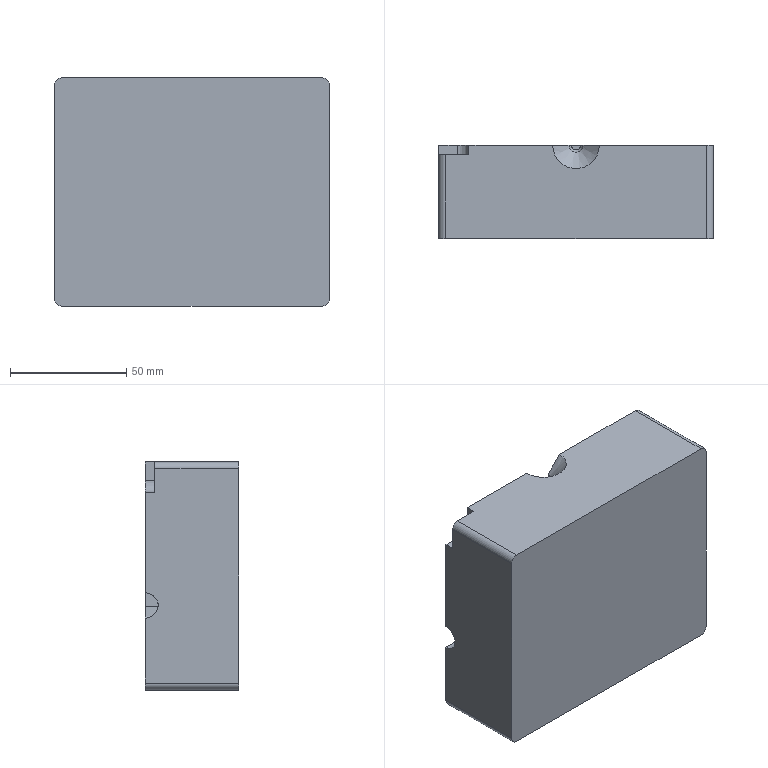NC program | NX | posted with a generic post | part box 118 x 40 x 98 mm
Lines 1 to 1487 of 39656, first 1399 of 1483 lines:
N10 G17 G21 G94 G90
(CAVITY_MILL , TOOL : D8)
N12 T00 M6
N14 G54
N16 G17 G0 G90 X63. Y44.15 S0 M3
N18 G43 Z30. H0
N20 Z-0.963
N22 G94 G1 X59. F250.
N24 X54.15
N26 Y49.
N28 X50.15
N30 Y41.
N32 G3 X51. Y40.15 R0.85
N34 G1 X59.
N36 X63.
N38 G0 Y44.15 Z-1.925
N40 G1 X59.
N42 X54.15
N44 Y49.
N46 X50.15
N48 Y41.
N50 G3 X51. Y40.15 R0.85
N52 G1 X59.
N54 X63.
N56 G0 Y44.15 Z-2.888
N58 G1 X59.
N60 X54.15
N62 Y49.
N64 X50.15
N66 Y41.
N68 G3 X51. Y40.15 R0.85
N70 G1 X59.
N72 X63.
N74 G0 Y44.15 Z-3.85
N76 G1 X59.
N78 X54.15
N80 Y49.
N82 X50.15
N84 Y41.
N86 G3 X51. Y40.15 R0.85
N88 G1 X59.
N90 X63.
N92 G0 Z30.
N94 X27.069 Y53.
N96 Z-0.963
N98 G1 Y49.
N100 Y5.639
N102 G2 X28.646 Y2.381 R4.133
N104 G1 Y-3.614
N106 X28.651 Y-3.624
N108 G2 X27.861 Y-6.049 R4.204
N110 X30.742 Y-10.011 R4.141
N112 G1 Y-17.85
N114 X31.058
N116 Y-10.
N118 G2 X33.939 Y-6.048 R4.142
N120 X33.154 Y-3.593 R4.131
N122 G1 Y2.381
N124 G2 X34.731 Y5.648 R4.173
N126 G1 Y49.
N128 Y53.
N130 G0 X27.248 Z-1.925
N132 G1 Y49.
N134 Y5.674
N136 G2 X28.872 Y2.372 R4.122
N138 G1 Y-3.614
N140 G2 X28.105 Y-6.02 R4.108
N142 X30.898 Y-8.748 R4.14
N144 X33.696 Y-6.02 R4.161
N146 X32.922 Y-3.631 R4.13
N148 G1 X32.928 Y-3.614
N150 Y2.362
N152 X32.922 Y2.376
N154 G2 X34.552 Y5.675 R4.162
N156 G1 Y48.627
N158 X34.548 Y48.99
N160 Y49.
N162 X34.549 Y53.
N164 G0 X27.557 Z-2.888
N166 G1 Y49.
N168 Y5.738
N170 G2 X29.27 Y2.372 R4.12
N172 G1 Y-3.614
N174 G2 X28.54 Y-5.964 R4.112
N176 X30.898 Y-7.482 R4.192
N178 X33.262 Y-5.964 R4.21
N180 X32.53 Y-3.614 R4.061
N182 G1 Y2.47
N184 G2 X32.736 Y3.675 R3.636
N186 X34.243 Y5.737 R4.091
N188 G1 Y48.627
N190 X34.244 Y49.
N192 X34.263 Y53.002
N194 G0 X28.029 Y53. Z-3.85
N196 G1 X28.013 Y49.
N198 X28.012 Y48.627
N200 Y5.84
N202 G2 X29.877 Y2.372 R4.129
N204 G1 Y-3.614
N206 G2 X29.204 Y-5.874 R4.028
N208 X30.9 Y-6.397 R4.605
N210 X32.594 Y-5.873 R4.686
N212 X31.923 Y-3.614 R4.073
N214 G1 Y2.372
N216 G2 X33.788 Y5.836 R4.116
N218 G1 Y49.
N220 Y53.
N222 G0 X28.649 Z-4.814
N224 G1 Y49.
N226 Y5.999
N228 G2 X30.794 Y2.372 R4.127
N230 G1 Y-3.614
N232 G2 X30.135 Y-5.85 R3.962
N234 G1 X31.665
N236 G2 X31.006 Y-3.614 R4.063
N238 G1 Y2.372
N240 G2 X33.151 Y5.997 R4.118
N242 G1 Y49.
N244 Y53.
N246 G0 X29.528 Z-5.778
N248 G1 Y49.
N250 Y6.271
N252 G2 X30.898 Y5.473 R4.416
N254 X32.272 Y6.27 R4.304
N256 G1 Y49.
N258 Y53.
N260 G0 X30.838 Z-6.742
N262 G1 X30.802 Y49.
N264 Y48.991
N266 Y6.625
N268 X30.998
N270 Y48.991
N272 Y49.
N274 X30.972 Y53.
N276 G0 Z30.
N278 X-34.726
N280 Z-0.963
N282 G1 X-34.731 Y49.
N284 Y18.094
N286 G2 X-34.817 Y17.17 R4.141
N288 G1 X-30.9 Y16.358
N290 G2 X-32.736 Y12.659 R8.141
N292 X-30.901 Y8.966 R8.142
N294 X-29.063 Y12.659 R8.158
N296 X-30.9 Y16.358 R8.143
N298 G1 X-34.817 Y17.17
N300 G2 X-38.868 Y13.869 R4.141
N302 G1 X-59.
N304 X-63.
N306 Y11.455
N308 X-59. Y11.451
N310 X-58.998
N312 X-38.907
N314 G2 X-34.731 Y7.302 R4.142
N316 G1 Y5.638
N318 G2 X-33.154 Y2.371 R4.167
N320 G1 Y-3.593
N322 G2 X-33.939 Y-6.048 R4.131
N324 X-31.058 Y-10. R4.142
N326 G1 Y-17.85
N328 X-30.742
N330 Y-10.
N332 G2 X-27.861 Y-6.049 R4.141
N334 X-28.651 Y-3.624 R4.212
N336 G1 X-28.646 Y-3.614
N338 Y2.33
N340 G2 X-27.069 Y5.627 R4.13
N342 G1 Y7.3
N344 G2 X-27.028 Y7.916 R4.615
N346 X-22.945 Y11.454 R4.158
N348 G1 X-22.932 Y11.451
N350 X-17.406
N352 G2 X-14.008 Y9.732 R4.144
N354 G1 X-10.765 Y12.074
N356 X-6.015 Y11.618
N358 X-1.702 Y11.205
N360 G2 X-1.232 Y6.796 R16.144
N362 G1 X-1.269 Y5.593
N364 G2 X0. Y5.208 R17.18
N366 X1.269 Y5.593 R17.18
N368 G1 X1.051 Y12.692
N370 G3 X-0.997 Y12.992 R1.051
N372 G2 X-1.702 Y11.205 R16.134
N374 G1 X-6.015 Y11.618
N376 G2 X-5.23 Y6.92 R12.144
N378 G1 X-5.377 Y2.148
N380 G2 X0. Y0.897 R13.18
N382 X5.377 Y2.148 R13.18
N384 G1 X5.049 Y12.815
N386 G3 X-4.797 Y14.24 R5.051
N388 G2 X-6.015 Y11.618 R12.134
N390 G1 X-10.765 Y12.074
N392 G2 X-9.228 Y7.046 R8.144
N394 G1 X-9.487 Y-1.369
N396 G2 X-9.512 Y-1.85 R10.725
N398 G1 X-5.61
N400 G2 X0. Y-3.764 R9.18
N402 X5.61 Y-1.85 R9.18
N404 G1 X9.512
N406 G2 X9.487 Y-1.369 R10.725
N408 G1 X9.047 Y12.938
N410 G3 X-8.599 Y15.485 R9.051
N412 G2 X-10.765 Y12.074 R8.134
N414 G1 X-14.008 Y9.732
N416 G2 X-13.226 Y7.172 R4.144
N418 G1 X-13.485 Y-1.246
N420 G2 X-15.508 Y-5.85 R6.725
N422 G1 X-5.61
N424 G2 X-0.525 Y-12.018 R5.18
N426 G1 X-3.027 Y-24.888
N428 X-1.75
N430 G2 X0. Y-25.269 R4.155
N432 X1.751 Y-24.888 R4.178
N434 G1 X3.027
N436 X0.525 Y-12.018
N438 G2 X5.61 Y-5.85 R5.18
N440 G1 X15.508
N442 G2 X13.485 Y-1.246 R6.725
N444 G1 X13.045 Y13.061
N446 G3 X-12.401 Y16.727 R13.051
N448 G2 X-16.352 Y13.869 R4.134
N450 G1 X-22.932
N452 G2 X-27.069 Y18.094 R4.143
N454 G1 Y49.
N456 Y53.
N458 G0 X-34.542 Z-1.925
N460 G1 X-34.552 Y49.
N462 Y18.094
N464 X-34.551 Y17.754
N466 G2 X-34.728 Y16.533 R4.134
N468 G1 X-30.899 Y15.375
N470 G2 X-32.325 Y12.659 R8.134
N472 X-30.9 Y9.946 R8.135
N474 X-29.475 Y12.662 R8.133
N476 X-29.772 Y13.057 R8.36
N478 X-30.899 Y15.375 R8.194
N480 G1 X-34.728 Y16.533
N482 G2 X-38.673 Y13.595 R4.134
N484 G1 X-59.
N486 X-63.
N488 Y11.727
N490 X-59. Y11.725
N492 X-58.993
N494 X-38.687
N496 G2 X-34.552 Y7.589 R4.135
N498 G1 Y5.664
N500 G2 X-32.928 Y2.371 R4.126
N502 G1 Y-3.614
N504 X-32.922 Y-3.631
N506 G2 X-33.695 Y-6.019 R4.131
N508 X-30.902 Y-8.75 R4.141
N510 X-28.105 Y-6.02 R4.157
N512 X-28.872 Y-3.614 R4.111
N514 G1 Y2.362
N516 G2 X-27.248 Y5.663 R4.117
N518 G1 Y7.592
N520 G2 X-23.116 Y11.725 R4.133
N522 G1 X-17.391
N524 G2 X-13.906 Y9.869 R4.147
N526 G1 X-10.572 Y12.08
N528 X-5.919 Y11.653
N530 X-1.641 Y11.26
N532 G2 X-1.224 Y7.055 R16.147
N534 G1 X-1.269 Y5.597
N536 G2 X0.004 Y5.213 R17.18
N538 X1.269 Y5.595 R17.187
N540 G1 X1.051 Y12.692
N542 G3 X-1.002 Y12.976 R1.051
N544 G2 X-1.641 Y11.26 R16.147
N546 G1 X-5.919 Y11.653
N548 G2 X-5.222 Y7.182 R12.147
N550 G1 X-5.377 Y2.148
N552 G2 X0.004 Y0.903 R13.18
N554 X5.377 Y2.148 R13.187
N556 G1 X5.049 Y12.815
N558 G3 X-4.822 Y14.162 R5.051
N560 G2 X-5.919 Y11.653 R12.147
N562 G1 X-10.572 Y12.08
N564 G2 X-9.22 Y7.309 R8.147
N566 G1 X-9.487 Y-1.369
N568 G2 X-9.512 Y-1.85 R10.725
N570 G1 X-5.593
N572 G2 X0.003 Y-3.753 R9.18
N574 X5.59 Y-1.85 R9.187
N576 G1 X9.512
N578 G2 X9.487 Y-1.369 R10.725
N580 G1 X9.047 Y12.938
N582 G3 X-8.644 Y15.345 R9.051
N584 G2 X-10.572 Y12.08 R8.147
N586 G1 X-13.906 Y9.869
N588 G2 X-13.218 Y7.437 R4.147
N590 G1 X-13.485 Y-1.246
N592 G2 X-15.508 Y-5.85 R6.725
N594 G1 X-5.593
N596 G2 X-0.508 Y-12.018 R5.18
N598 G1 X-3.006 Y-24.871
N600 X-0.532
N602 X-0.174 Y-24.879
N604 X0. Y-24.89
N606 G2 X0.529 Y-24.871 R5.99
N608 G1 X3.006
N610 X0.511 Y-12.036
N612 G2 X5.593 Y-5.85 R5.187
N614 G1 X15.508
N616 G2 X13.485 Y-1.246 R6.725
N618 G1 X13.045 Y13.061
N620 G3 X-12.465 Y16.526 R13.051
N622 G2 X-16.436 Y13.595 R4.147
N624 G1 X-23.119
N626 G2 X-25.166 Y14.136 R4.14
N628 X-26.502 Y15.36 R4.36
N630 X-27.246 Y17.528 R4.194
N632 G1 X-27.248 Y18.094
N634 Y49.
N636 Y53.
N638 G0 X-34.243 Z-2.888
N640 G1 Y49.
N642 Y17.237
N644 G2 X-34.485 Y15.832 R4.195
N646 X-34.576 Y15.599 R4.12
N648 G1 X-30.899 Y14.025
N650 G2 X-31.647 Y12.659 R8.12
N652 X-30.901 Y11.295 R8.131
N654 X-30.153 Y12.661 R8.123
N656 X-30.899 Y14.025 R8.133
N658 G1 X-34.576 Y15.599
N660 G2 X-38.401 Y13.101 R4.12
N662 G1 X-59.
N664 X-63.
N666 Y12.219
N668 X-59.
N670 X-38.907
N672 X-38.343 Y12.222
N674 G2 X-34.243 Y8.076 R4.131
N676 G1 Y5.728
N678 G2 X-32.838 Y3.958 R4.254
N680 G1 X-32.698 Y3.537
N682 G2 X-32.53 Y2.499 R3.292
N684 G1 Y-3.614
N686 G2 X-33.261 Y-5.964 R4.061
N688 X-30.902 Y-7.482 R4.17
N690 X-28.544 Y-5.965 R4.243
N692 X-29.27 Y-3.614 R4.166
N694 G1 Y2.362
N696 G2 X-27.557 Y5.727 R4.119
N698 G1 Y8.077
N700 G2 X-23.395 Y12.219 R4.123
N702 G1 X-17.313
N704 G2 X-13.815 Y10.235 R4.119
N706 G1 X-13.783 Y10.178
N708 X-13.75 Y10.12
N710 X-10.272 Y12.097
N712 X-5.766 Y11.715
N714 X-1.543 Y11.358
N716 G2 X-1.209 Y7.542 R16.2
N718 G1 X-1.269 Y5.601
N720 G2 X0.004 Y5.219 R17.18
N722 X1.269 Y5.599 R17.187
N724 G1 X1.051 Y12.692
N726 G3 X-1.012 Y12.943 R1.051
N728 G2 X-1.543 Y11.358 R16.201
N730 G1 X-5.766 Y11.715
N732 G2 X-5.207 Y7.666 R12.2
N734 G1 X-5.377 Y2.148
N736 G2 X0.004 Y0.911 R13.18
N738 X5.377 Y2.148 R13.187
N740 G1 X5.049 Y12.815
N742 G3 X-4.865 Y14.018 R5.051
N744 G2 X-5.766 Y11.715 R12.201
N746 G1 X-10.272 Y12.097
N748 G2 X-9.205 Y7.79 R8.2
N750 G1 X-9.487 Y-1.369
N752 G2 X-9.512 Y-1.85 R10.725
N754 G1 X-5.576
N756 G2 X0.003 Y-3.74 R9.18
N758 X5.572 Y-1.85 R9.187
N760 G1 X9.512
N762 G2 X9.487 Y-1.369 R10.725
N764 G1 X9.047 Y12.938
N766 G3 X-8.718 Y15.091 R9.051
N768 G2 X-10.272 Y12.097 R8.201
N770 G1 X-13.75 Y10.12
N772 G2 X-13.203 Y7.914 R4.2
N774 G1 X-13.485 Y-1.246
N776 G2 X-15.508 Y-5.85 R6.725
N778 G1 X-5.576
N780 G2 X-0.491 Y-12.018 R5.18
N782 G1 X-2.986 Y-24.855
N784 X2.986
N786 X0.494 Y-12.036
N788 G2 X5.576 Y-5.85 R5.187
N790 G1 X15.508
N792 G2 X13.485 Y-1.246 R6.725
N794 G1 X13.045 Y13.061
N796 G3 X-12.572 Y16.164 R13.051
N798 G2 X-16.07 Y13.125 R4.201
N800 G1 X-16.596 Y13.094
N802 X-16.614 Y13.101
N804 X-23.44
N806 G2 X-25.703 Y13.781 R4.105
N808 X-27.557 Y17.229 R4.133
N810 G1 Y49.
N812 Y53.
N814 G0 Z30.
N816 X-2.563 Y12.197
N818 Z-2.388
N820 G3 X-2.563 Y12.197 Z-2.607 I1.979 J-0.286
N822 X-2.563 Y12.197 Z-2.826 I1.979 J-0.286
N824 X-2.563 Y12.197 Z-3.046 I1.979 J-0.286
N826 X-2.563 Y12.197 Z-3.265 I1.979 J-0.286
N828 X-2.563 Y12.197 Z-3.484 I1.979 J-0.286
N830 X-2.563 Y12.197 Z-3.704 I1.979 J-0.286
N832 X0.646 Y13.489 Z-3.85 R-2.
N834 X-0.473 Y13.598 R1.051
N836 X-1.027 Y12.883 R1.051
N838 G2 X-1.407 Y11.517 R16.402
N840 X-1.184 Y8.341 R16.452
N842 G1 X-1.269 Y5.606
N844 G2 X0.004 Y5.225 R17.18
N846 X1.269 Y5.604 R17.187
N848 G1 X1.051 Y12.692
N850 G3 X0.646 Y13.489 R1.051
N852 G1 X3.104 Y16.645
N854 G3 X-2.274 Y17.17 R5.051
N856 X-4.925 Y13.779 R5.051
N858 G2 X-5.555 Y11.824 R12.402
N860 X-5.183 Y8.456 R12.452
N862 G1 X-5.377 Y2.149
N864 G2 X0.004 Y0.919 R13.18
N866 X5.377 Y2.149 R13.187
N868 G1 X5.049 Y12.815
N870 G3 X3.104 Y16.645 R5.051
N872 G1 X5.562 Y19.801
N874 G3 X-8.823 Y14.68 R9.051
N876 G2 X-9.876 Y12.144 R8.402
N878 X-9.603 Y11.429 R8.123
N880 X-9.181 Y8.568 R8.452
N882 G1 X-9.487 Y-1.369
N884 G2 X-9.512 Y-1.85 R10.725
N886 G1 X-5.559
N888 G2 X0.003 Y-3.727 R9.18
N890 X5.555 Y-1.85 R9.187
N892 G1 X9.512
N894 G2 X9.487 Y-1.369 R10.725
N896 G1 X9.047 Y12.938
N898 G3 X5.562 Y19.801 R9.051
N900 G1 X8.02 Y22.956
N902 G3 X-12.719 Y15.585 R13.051
N904 G2 X-13.533 Y13.884 R4.402
N906 X-15.407 Y12.542 R4.123
N908 X-13.402 Y10.178 R4.123
N910 X-13.18 Y8.678 R4.452
N912 G1 X-13.485 Y-1.246
N914 G2 X-15.508 Y-5.85 R6.725
N916 G1 X-5.559
N918 G2 X-0.474 Y-12.018 R5.18
N920 G1 X-2.966 Y-24.838
N922 X2.966
N924 X0.477 Y-12.036
N926 G2 X5.559 Y-5.85 R5.187
N928 G1 X15.508
N930 G2 X13.485 Y-1.246 R6.725
N932 G1 X13.045 Y13.061
N934 G3 X8.02 Y22.956 R13.051
N936 G1 X7.036 Y21.694
N938 G0 X-2.547 Y12.291 Z-3.35
N940 G3 X-2.547 Y12.291 Z-3.569 I1.964 J-0.38
N942 X-2.547 Y12.291 Z-3.789 I1.964 J-0.38
N944 X-2.547 Y12.291 Z-4.008 I1.964 J-0.38
N946 X-2.547 Y12.291 Z-4.227 I1.964 J-0.38
N948 X-2.547 Y12.291 Z-4.447 I1.964 J-0.38
N950 X-2.547 Y12.291 Z-4.666 I1.964 J-0.38
N952 X0.646 Y13.489 Z-4.814 R-2.
N954 X-1.039 Y12.818 R1.051
N956 G2 X-1.221 Y11.81 R16.601
N958 X-1.146 Y9.601 R16.541
N960 G1 X-1.268 Y5.61
N962 G2 X0.004 Y5.23 R17.18
N964 X1.268 Y5.608 R17.187
N966 G1 X1.051 Y12.692
N968 G3 X0.646 Y13.489 R1.051
N970 G1 X3.104 Y16.645
N972 G3 X-4.995 Y13.411 R5.051
N974 G2 X-5.28 Y12.03 R12.601
N976 X-5.144 Y9.728 R12.541
N978 G1 X-5.377 Y2.149
N980 G2 X0.004 Y0.927 R13.18
N982 X5.377 Y2.149 R13.187
N984 G1 X5.049 Y12.815
N986 G3 X3.104 Y16.645 R5.051
N988 G1 X5.562 Y19.801
N990 G3 X-8.951 Y14.002 R9.051
N992 G2 X-9.403 Y12.253 R8.601
N994 X-9.142 Y9.855 R8.541
N996 G1 X-9.487 Y-1.369
N998 G2 X-9.512 Y-1.85 R10.725
N1000 G1 X-5.542
N1002 G2 X0.003 Y-3.714 R9.18
N1004 X5.538 Y-1.85 R9.187
N1006 G1 X9.512
N1008 G2 X9.487 Y-1.369 R10.725
N1010 G1 X9.047 Y12.938
N1012 G3 X5.562 Y19.801 R9.051
N1014 G1 X8.02 Y22.956
N1016 G3 X-12.907 Y14.592 R13.051
N1018 G2 X-13.791 Y12.488 R4.601
N1020 X-13.139 Y9.984 R4.541
N1022 G1 X-13.485 Y-1.246
N1024 G2 X-15.508 Y-5.85 R6.725
N1026 G1 X-5.542
N1028 G2 X-0.457 Y-12.018 R5.18
N1030 G1 X-2.945 Y-24.821
N1032 X2.945
N1034 X0.46 Y-12.036
N1036 G2 X5.542 Y-5.85 R5.187
N1038 G1 X15.508
N1040 G2 X13.485 Y-1.246 R6.725
N1042 G1 X13.045 Y13.061
N1044 G3 X8.02 Y22.956 R13.051
N1046 G1 X7.036 Y21.694
N1048 G0 X-2.547 Y12.291 Z-4.314
N1050 G3 X-2.547 Y12.291 Z-4.534 I1.964 J-0.38
N1052 X-2.547 Y12.291 Z-4.753 I1.964 J-0.38
N1054 X-2.547 Y12.291 Z-4.972 I1.964 J-0.38
N1056 X-2.547 Y12.291 Z-5.192 I1.964 J-0.38
N1058 X-2.547 Y12.291 Z-5.411 I1.964 J-0.38
N1060 X-2.547 Y12.291 Z-5.63 I1.964 J-0.38
N1062 X0.646 Y13.489 Z-5.778 R-2.
N1064 X-1.051 Y12.692 R1.051
N1066 G1 X-1.268 Y5.614
N1068 G2 X0.004 Y5.236 R17.18
N1070 X1.268 Y5.612 R17.187
N1072 G1 X1.051 Y12.692
N1074 G3 X0.646 Y13.489 R1.051
N1076 G1 X3.104 Y16.645
N1078 G3 X-5.049 Y12.815 R5.051
N1080 G1 X-5.377 Y2.149
N1082 G2 X0.004 Y0.935 R13.18
N1084 X5.377 Y2.149 R13.187
N1086 G1 X5.049 Y12.815
N1088 G3 X3.104 Y16.645 R5.051
N1090 G1 X5.562 Y19.801
N1092 G3 X-9.047 Y12.938 R9.051
N1094 G1 X-9.487 Y-1.369
N1096 G2 X-9.512 Y-1.85 R10.725
N1098 G1 X-5.524
N1100 G2 X0.003 Y-3.701 R9.18
N1102 X5.521 Y-1.85 R9.187
N1104 G1 X9.512
N1106 G2 X9.487 Y-1.369 R10.725
N1108 G1 X9.047 Y12.938
N1110 G3 X5.562 Y19.801 R9.051
N1112 G1 X8.02 Y22.956
N1114 G3 X-13.045 Y13.061 R13.051
N1116 G1 X-13.485 Y-1.246
N1118 G2 X-15.508 Y-5.85 R6.725
N1120 G1 X-5.524
N1122 G2 X-0.439 Y-12.018 R5.18
N1124 G1 X-2.925 Y-24.804
N1126 X2.925
N1128 X0.443 Y-12.036
N1130 G2 X5.524 Y-5.85 R5.187
N1132 G1 X15.508
N1134 G2 X13.485 Y-1.246 R6.725
N1136 G1 X13.045 Y13.061
N1138 G3 X8.02 Y22.956 R13.051
N1140 G1 X7.036 Y21.694
N1142 G0 X-2.547 Y12.291 Z-5.278
N1144 G3 X-2.547 Y12.291 Z-5.498 I1.964 J-0.38
N1146 X-2.547 Y12.291 Z-5.717 I1.964 J-0.38
N1148 X-2.547 Y12.291 Z-5.936 I1.964 J-0.38
N1150 X-2.547 Y12.291 Z-6.156 I1.964 J-0.38
N1152 X-2.547 Y12.291 Z-6.375 I1.964 J-0.38
N1154 X-2.547 Y12.291 Z-6.594 I1.964 J-0.38
N1156 X0.646 Y13.489 Z-6.742 R-2.
N1158 X-1.051 Y12.692 R1.051
N1160 G1 X-1.268 Y5.619
N1162 G2 X0.004 Y5.242 R17.18
N1164 X1.268 Y5.617 R17.187
N1166 G1 X1.051 Y12.692
N1168 G3 X0.646 Y13.489 R1.051
N1170 G1 X3.104 Y16.645
N1172 G3 X-5.049 Y12.815 R5.051
N1174 G1 X-5.377 Y2.149
N1176 G2 X0.004 Y0.943 R13.18
N1178 X5.377 Y2.149 R13.187
N1180 G1 X5.049 Y12.815
N1182 G3 X3.104 Y16.645 R5.051
N1184 G1 X5.562 Y19.801
N1186 G3 X-9.047 Y12.938 R9.051
N1188 G1 X-9.487 Y-1.369
N1190 G2 X-9.512 Y-1.85 R10.725
N1192 G1 X-5.507
N1194 G2 X0.003 Y-3.688 R9.18
N1196 X5.504 Y-1.85 R9.187
N1198 G1 X9.512
N1200 G2 X9.487 Y-1.369 R10.725
N1202 G1 X9.047 Y12.938
N1204 G3 X5.562 Y19.801 R9.051
N1206 G1 X8.02 Y22.956
N1208 G3 X-13.045 Y13.061 R13.051
N1210 G1 X-13.485 Y-1.246
N1212 G2 X-15.508 Y-5.85 R6.725
N1214 G1 X-5.507
N1216 G2 X-0.422 Y-12.018 R5.18
N1218 G1 X-2.904 Y-24.787
N1220 X2.904
N1222 X0.426 Y-12.036
N1224 G2 X5.507 Y-5.85 R5.187
N1226 G1 X15.508
N1228 G2 X13.485 Y-1.246 R6.725
N1230 G1 X13.045 Y13.061
N1232 G3 X8.02 Y22.956 R13.051
N1234 G1 X7.036 Y21.694
N1236 G0 X-2.547 Y12.291 Z-6.242
N1238 G3 X-2.547 Y12.291 Z-6.462 I1.964 J-0.38
N1240 X-2.547 Y12.291 Z-6.681 I1.964 J-0.38
N1242 X-2.547 Y12.291 Z-6.901 I1.964 J-0.38
N1244 X-2.547 Y12.291 Z-7.12 I1.964 J-0.38
N1246 X-2.547 Y12.291 Z-7.339 I1.964 J-0.38
N1248 X-2.547 Y12.291 Z-7.559 I1.964 J-0.38
N1250 X0.646 Y13.489 Z-7.707 R-2.
N1252 X-1.051 Y12.692 R1.051
N1254 G1 X-1.268 Y5.625
N1256 G2 X0.002 Y5.25 R17.184
N1258 X1.268 Y5.623 R17.18
N1260 G1 X1.051 Y12.692
N1262 G3 X0.646 Y13.489 R1.051
N1264 G1 X3.104 Y16.645
N1266 G3 X-5.049 Y12.815 R5.051
N1268 G1 X-5.377 Y2.15
N1270 X-5.234
N1272 G2 X0.001 Y0.953 R13.184
N1274 X5.377 Y2.15 R13.18
N1276 G1 X5.049 Y12.815
N1278 G3 X3.104 Y16.645 R5.051
N1280 G1 X5.562 Y19.801
N1282 G3 X-9.047 Y12.938 R9.051
N1284 G1 X-9.487 Y-1.369
N1286 G2 X-9.512 Y-1.85 R10.725
N1288 G1 X-5.28
N1290 G2 X0. Y-3.673 R9.184
N1292 X5.49 Y-1.85 R9.18
N1294 G1 X9.512
N1296 G2 X9.487 Y-1.369 R10.725
N1298 G1 X9.047 Y12.938
N1300 G3 X5.562 Y19.801 R9.051
N1302 G1 X8.02 Y22.956
N1304 G3 X-13.045 Y13.061 R13.051
N1306 G1 X-13.485 Y-1.246
N1308 G2 X-15.508 Y-5.85 R6.725
N1310 G1 X-5.34
N1312 G2 X-0.405 Y-12.018 R5.184
N1314 G1 X-2.884 Y-24.77
N1316 X2.884
N1318 X0.405 Y-12.018
N1320 G2 X5.49 Y-5.85 R5.18
N1322 G1 X15.508
N1324 G2 X13.485 Y-1.246 R6.725
N1326 G1 X13.045 Y13.061
N1328 G3 X8.02 Y22.956 R13.051
N1330 G1 X7.036 Y21.694
N1332 G0 X-2.555 Y12.281 Z-7.207
N1334 G3 X-2.555 Y12.281 Z-7.426 I1.964 J-0.38
N1336 X-2.555 Y12.281 Z-7.645 I1.964 J-0.38
N1338 X-2.555 Y12.281 Z-7.865 I1.964 J-0.38
N1340 X-2.555 Y12.281 Z-8.084 I1.964 J-0.38
N1342 X-2.555 Y12.281 Z-8.303 I1.964 J-0.38
N1344 X-2.555 Y12.281 Z-8.523 I1.964 J-0.38
N1346 X0.638 Y13.479 Z-8.671 R-2.
N1348 X-1.037 Y12.692 R1.038
N1350 G1 X-1.255 Y5.627
N1352 G2 X0.001 Y5.257 R17.193
N1354 X1.255 Y5.626 R17.18
N1356 G1 X1.037 Y12.692
N1358 G3 X0.638 Y13.479 R1.038
N1360 G1 X3.096 Y16.634
N1362 G3 X-5.035 Y12.815 R5.038
N1364 G1 X-5.363 Y2.15
N1366 X-5.193
N1368 G2 X0. Y0.963 R13.193
N1370 X5.363 Y2.15 R13.18
N1372 G1 X5.035 Y12.815
N1374 G3 X3.096 Y16.634 R5.038
N1376 G1 X5.553 Y19.79
N1378 G3 X-9.033 Y12.938 R9.038
N1380 G1 X-9.473 Y-1.345
N1382 G2 X-9.496 Y-1.85 R10.004
N1384 G1 X-5.243
N1386 G2 X-0.001 Y-3.655 R9.193
N1388 X5.472 Y-1.85 R9.18
N1390 G1 X9.496
N1392 G2 X9.471 Y-1.367 R10.699
N1394 G1 X9.469 Y-1.217
N1396 X9.033 Y12.938
N1398 G3 X5.553 Y19.79 R9.038
N1400 G1 X8.011 Y22.946
N1402 G3 X-13.032 Y13.061 R13.038
N1404 G1 X-13.472 Y-1.245
N1406 G2 X-13.561 Y-2.175 R6.004
N1408 X-15.493 Y-5.85 R6.758
N1410 G1 X-5.308
N1412 G2 X-0.366 Y-11.968 R5.193
N1414 G1 X-0.383 Y-12.017
N1416 X-2.857 Y-24.749
N1418 X2.857
N1420 X0.402 Y-12.116
N1422 G2 X5.471 Y-5.85 R5.18
N1424 G1 X15.497
N1426 G2 X13.469 Y-1.247 R6.699
N1428 G1 X13.472 Y-1.245
N1430 X13.032 Y13.061
N1432 G3 X8.011 Y22.946 R13.038
N1434 G1 X7.028 Y21.684
N1436 G0 Z30.
N1438 X-0.383 Y-23.247
N1440 Z-8.171
N1442 G3 X-0.383 Y-23.247 Z-8.311 I0.383 J1.221
N1444 X-0.383 Y-23.247 Z-8.452 I0.383 J1.221
N1446 X-0.383 Y-23.247 Z-8.592 I0.383 J1.221
N1448 X-0.383 Y-23.247 Z-8.732 I0.383 J1.221
N1450 X-0.383 Y-23.247 Z-8.873 I0.383 J1.221
N1452 X-0.383 Y-23.247 Z-9.013 I0.383 J1.221
N1454 X-0.383 Y-23.247 Z-9.154 I0.383 J1.221
N1456 X-0.383 Y-23.247 Z-9.294 I0.383 J1.221
N1458 X-0.383 Y-23.247 Z-9.434 I0.383 J1.221
N1460 X-0.383 Y-23.247 Z-9.575 I0.383 J1.221
N1462 X0.868 Y-21.085 Z-9.635 R1.28
N1464 G1 X-0.819 Y-19.531
N1466 X-1.638 Y-23.743
N1468 X1.638
N1470 X0. Y-15.318
N1472 X-0.819 Y-19.531
N1474 X0.752 Y-19.836
N1476 G0 Z30.
N1478 X-2.801 Y11.965
N1480 Z-8.171
N1482 G3 X-2.801 Y11.965 Z-8.39 I1.964 J-0.38
N1484 X-2.801 Y11.965 Z-8.61 I1.964 J-0.38
N1486 X-2.801 Y11.965 Z-8.829 I1.964 J-0.38
N1488 X-2.801 Y11.965 Z-9.048 I1.964 J-0.38
N1490 X-2.801 Y11.965 Z-9.268 I1.964 J-0.38
N1492 X-2.801 Y11.965 Z-9.487 I1.964 J-0.38
N1494 X0.392 Y13.163 Z-9.635 R-2.
N1496 X-0.637 Y12.68 R0.638
N1498 G1 X-0.855 Y5.609
N1500 G2 X0. Y5.37 R17.834
N1502 X0.855 Y5.609 R17.828
N1504 G1 X0.637 Y12.68
N1506 G3 X0.392 Y13.163 R0.638
N1508 G1 X2.85 Y16.319
N1510 G3 X-4.636 Y12.803 R4.638
N1512 G1 X-4.963 Y2.148
N1514 G2 X0. Y1.129 R13.834
N1516 X4.963 Y2.148 R13.828
N1518 G1 X4.636 Y12.803
N1520 G3 X2.85 Y16.319 R4.638
N1522 G1 X5.308 Y19.475
N1524 G3 X-8.634 Y12.926 R8.638
N1526 G1 X-9.086 Y-1.78
N1528 X-9.088 Y-1.85
N1530 X-5.186
N1532 G2 X-0.688 Y-2.954 R9.834
N1534 X0.001 Y-3.344 R11.752
N1536 X0.684 Y-2.956 R11.722
N1538 X5.185 Y-1.85 R9.828
N1540 G1 X9.088
N1542 X9.086 Y-1.778
N1544 X8.634 Y12.926
N1546 G3 X5.308 Y19.475 R8.638
N1548 G1 X7.766 Y22.63
N1550 G3 X-12.632 Y13.049 R12.638
N1552 G1 X-13.085 Y-1.68
N1554 G2 X-14.862 Y-5.85 R6.027
N1556 G1 X-5.193
N1558 G2 X-2.534 Y-6.502 R5.834
N1560 X0.007 Y-8.632 R7.752
N1562 X2.535 Y-6.502 R7.722
N1564 X5.192 Y-5.85 R5.828
N1566 G1 X14.864
N1568 G2 X13.085 Y-1.68 R6.012
N1570 G1 X12.632 Y13.049
N1572 G3 X7.766 Y22.63 R12.638
N1574 G1 X6.782 Y21.368
N1576 G0 X0.4 Y6.509 Z-9.135
N1578 G3 X0.4 Y6.509 Z-9.354 I-1.802 J0.868
N1580 X0.4 Y6.509 Z-9.574 I-1.802 J0.868
N1582 X0.4 Y6.509 Z-9.793 I-1.802 J0.868
N1584 X0.4 Y6.509 Z-10.012 I-1.802 J0.868
N1586 X0.4 Y6.509 Z-10.232 I-1.802 J0.868
N1588 X-3.401 Y7.438 Z-10.356 R-2.
N1590 G1 X-3.565 Y2.117
N1592 G2 X-2.825 Y2.058 R19.124
N1594 G1 X-0.002 Y2.057
N1596 X2.838 Y2.059
N1598 G2 X3.565 Y2.117 R19.215
N1600 G1 X3.237 Y12.76
N1602 G3 X-3.237 Y12.76 R3.239
N1604 G1 X-3.401 Y7.438
N1606 X-7.399 Y7.561
N1608 X-7.688 Y-1.85
N1610 X-4.535
N1612 G2 X-3.059 Y-1.939 R15.124
N1614 G1 X-3.004 Y-1.942
N1616 X-0.001 Y-1.943
N1618 X3.012 Y-1.941
N1620 X3.069 Y-1.938
N1622 G2 X4.534 Y-1.85 R15.215
N1624 G1 X7.688
N1626 X7.235 Y12.883
N1628 G3 X-7.235 Y12.883 R7.239
N1630 G1 X-7.399 Y7.561
N1632 X-11.397 Y7.684
N1634 X-11.728 Y-3.069
N1636 G2 X-12.88 Y-5.85 R4.292
N1638 G1 X-4.561
N1640 G2 X-3.383 Y-5.928 R11.124
N1642 G1 X-3.102 Y-5.942
N1644 X0. Y-5.943
N1646 X3.102 Y-5.941
N1648 X3.383 Y-5.928
N1650 G2 X4.561 Y-5.85 R11.215
N1652 G1 X12.873
N1654 G2 X11.728 Y-3.069 R4.164
N1656 G1 X11.233 Y13.006
N1658 G3 X-11.233 Y13.006 R11.239
N1660 G1 X-11.397 Y7.684
N1662 X-9.798 Y7.635
N1664 G0 Z30.
N1666 X-33.788 Y53.
N1668 Z-3.85
N1670 G1 Y49.
N1672 Y16.441
N1674 G2 X-36.224 Y12.661 R4.113
N1676 X-33.836 Y9.506 R4.097
N1678 X-33.788 Y8.839 R4.657
N1680 G1 Y5.829
N1682 G2 X-31.923 Y2.362 R4.126
N1684 G1 Y-3.614
N1686 G2 X-32.594 Y-5.874 R4.077
N1688 X-30.9 Y-6.397 R4.674
N1690 X-29.207 Y-5.875 R4.643
N1692 X-29.877 Y-3.614 R4.069
N1694 G1 Y2.362
N1696 G2 X-28.012 Y5.826 R4.112
N1698 G1 Y8.806
N1700 G2 X-27.918 Y9.748 R4.772
N1702 X-25.576 Y12.658 R4.052
N1704 X-27.989 Y16.049 R4.094
N1706 X-28.012 Y16.58 R6.243
N1708 G1 Y49.
N1710 Y53.
N1712 G0 X-33.151 Z-4.814
N1714 G1 Y49.
N1716 Y15.027
N1718 G2 X-33.866 Y12.66 R4.229
N1720 X-33.151 Y10.292 R4.218
N1722 G1 Y5.991
N1724 G2 X-31.006 Y2.362 R4.139
N1726 G1 Y-3.614
N1728 G2 X-31.665 Y-5.85 R4.063
N1730 G1 X-30.135
N1732 G2 X-30.794 Y-3.614 R3.964
N1734 G1 Y2.362
N1736 G2 X-28.649 Y5.99 R4.13
N1738 G1 Y10.293
N1740 G2 X-27.933 Y12.66 R4.252
N1742 X-28.649 Y15.028 R4.254
N1744 G1 Y49.
N1746 Y53.
N1748 G0 X-32.272 Z-5.778
N1750 G1 Y49.
N1752 Y6.259
N1754 G2 X-30.9 Y5.462 R4.151
N1756 X-29.528 Y6.259 R4.357
N1758 G1 Y49.
N1760 Y53.
N1762 G0 X-30.998 Z-6.742
N1764 G1 Y49.
N1766 Y6.615
N1768 X-30.802
N1770 Y49.
N1772 Y53.
N1774 G0 Z30.
N1776 X-50.75 Y38.985
N1778 Z0.5
N1780 G3 X-50.75 Y38.985 Z0.308 I1.75 J0.015
N1782 X-50.75 Y38.985 Z0.116 I1.75 J0.015
N1784 X-50.75 Y38.985 Z-0.076 I1.75 J0.015
N1786 X-50.75 Y38.985 Z-0.268 I1.75 J0.015
N1788 X-50.75 Y38.985 Z-0.46 I1.75 J0.015
N1790 X-50.75 Y38.985 Z-0.652 I1.75 J0.015
N1792 X-50.75 Y38.985 Z-0.844 I1.75 J0.015
N1794 X-47.735 Y40.209 Z-0.963 R-1.75
N1796 X-50.209 Y40.265 R1.75
N1798 X-47.735 Y40.209 R-1.75
N1800 G1 X-48.892 Y39.104
N1802 G0 X-50.75 Y38.985 Z-0.463
N1804 G3 X-50.75 Y38.985 Z-0.654 I1.75 J0.015
N1806 X-50.75 Y38.985 Z-0.846 I1.75 J0.015
N1808 X-50.75 Y38.985 Z-1.038 I1.75 J0.015
N1810 X-50.75 Y38.985 Z-1.23 I1.75 J0.015
N1812 X-50.75 Y38.985 Z-1.422 I1.75 J0.015
N1814 X-50.75 Y38.985 Z-1.614 I1.75 J0.015
N1816 X-50.75 Y38.985 Z-1.806 I1.75 J0.015
N1818 X-47.735 Y40.209 Z-1.925 R-1.75
N1820 X-50.209 Y40.265 R1.75
N1822 X-47.735 Y40.209 R-1.75
N1824 G1 X-48.892 Y39.104
N1826 G0 X-50.75 Y38.985 Z-1.425
N1828 G3 X-50.75 Y38.985 Z-1.617 I1.75 J0.015
N1830 X-50.75 Y38.985 Z-1.809 I1.75 J0.015
N1832 X-50.75 Y38.985 Z-2.001 I1.75 J0.015
N1834 X-50.75 Y38.985 Z-2.193 I1.75 J0.015
N1836 X-50.75 Y38.985 Z-2.385 I1.75 J0.015
N1838 X-50.75 Y38.985 Z-2.577 I1.75 J0.015
N1840 X-50.75 Y38.985 Z-2.769 I1.75 J0.015
N1842 X-47.735 Y40.209 Z-2.888 R-1.75
N1844 X-50.209 Y40.265 R1.75
N1846 X-47.735 Y40.209 R-1.75
N1848 G1 X-48.892 Y39.104
N1850 G0 X-50.75 Y38.985 Z-2.388
N1852 G3 X-50.75 Y38.985 Z-2.579 I1.75 J0.015
N1854 X-50.75 Y38.985 Z-2.771 I1.75 J0.015
N1856 X-50.75 Y38.985 Z-2.963 I1.75 J0.015
N1858 X-50.75 Y38.985 Z-3.155 I1.75 J0.015
N1860 X-50.75 Y38.985 Z-3.347 I1.75 J0.015
N1862 X-50.75 Y38.985 Z-3.539 I1.75 J0.015
N1864 X-50.75 Y38.985 Z-3.731 I1.75 J0.015
N1866 X-47.735 Y40.209 Z-3.85 R-1.75
N1868 X-50.209 Y40.265 R1.75
N1870 X-47.735 Y40.209 R-1.75
N1872 G1 X-48.892 Y39.104
N1874 G0 X-50.748 Y39.08 Z-3.35
N1876 G3 X-50.748 Y39.08 Z-3.542 I1.748 J-0.08
N1878 X-50.748 Y39.08 Z-3.734 I1.748 J-0.08
N1880 X-50.748 Y39.08 Z-3.926 I1.748 J-0.08
N1882 X-50.748 Y39.08 Z-4.118 I1.748 J-0.08
N1884 X-50.748 Y39.08 Z-4.31 I1.748 J-0.08
N1886 X-50.748 Y39.08 Z-4.502 I1.748 J-0.08
N1888 X-50.748 Y39.08 Z-4.694 I1.748 J-0.08
N1890 X-47.735 Y40.209 Z-4.814 R-1.75
N1892 X-50.209 Y40.265 R1.75
N1894 X-47.735 Y40.209 R-1.75
N1896 G1 X-48.892 Y39.104
N1898 G0 X-50.748 Y39.08 Z-4.314
N1900 G3 X-50.748 Y39.08 Z-4.506 I1.748 J-0.08
N1902 X-50.748 Y39.08 Z-4.698 I1.748 J-0.08
N1904 X-50.748 Y39.08 Z-4.89 I1.748 J-0.08
N1906 X-50.748 Y39.08 Z-5.082 I1.748 J-0.08
N1908 X-50.748 Y39.08 Z-5.274 I1.748 J-0.08
N1910 X-50.748 Y39.08 Z-5.466 I1.748 J-0.08
N1912 X-50.748 Y39.08 Z-5.658 I1.748 J-0.08
N1914 X-47.735 Y40.209 Z-5.778 R-1.75
N1916 X-50.209 Y40.265 R1.75
N1918 X-47.735 Y40.209 R-1.75
N1920 G1 X-48.892 Y39.104
N1922 G0 X-50.748 Y39.08 Z-5.278
N1924 G3 X-50.748 Y39.08 Z-5.47 I1.748 J-0.08
N1926 X-50.748 Y39.08 Z-5.662 I1.748 J-0.08
N1928 X-50.748 Y39.08 Z-5.854 I1.748 J-0.08
N1930 X-50.748 Y39.08 Z-6.046 I1.748 J-0.08
N1932 X-50.748 Y39.08 Z-6.238 I1.748 J-0.08
N1934 X-50.748 Y39.08 Z-6.43 I1.748 J-0.08
N1936 X-50.748 Y39.08 Z-6.622 I1.748 J-0.08
N1938 X-47.735 Y40.209 Z-6.742 R-1.75
N1940 X-50.209 Y40.265 R1.75
N1942 X-47.735 Y40.209 R-1.75
N1944 G1 X-48.892 Y39.104
N1946 G0 X-50.748 Y39.08 Z-6.242
N1948 G3 X-50.748 Y39.08 Z-6.434 I1.748 J-0.08
N1950 X-50.748 Y39.08 Z-6.626 I1.748 J-0.08
N1952 X-50.748 Y39.08 Z-6.818 I1.748 J-0.08
N1954 X-50.748 Y39.08 Z-7.01 I1.748 J-0.08
N1956 X-50.748 Y39.08 Z-7.202 I1.748 J-0.08
N1958 X-50.748 Y39.08 Z-7.394 I1.748 J-0.08
N1960 X-50.748 Y39.08 Z-7.586 I1.748 J-0.08
N1962 X-47.735 Y40.209 Z-7.707 R-1.75
N1964 X-50.209 Y40.265 R1.75
N1966 X-47.735 Y40.209 R-1.75
N1968 G1 X-48.892 Y39.104
N1970 G0 X-50.748 Y39.08 Z-7.207
N1972 G3 X-50.748 Y39.08 Z-7.399 I1.748 J-0.08
N1974 X-50.748 Y39.08 Z-7.591 I1.748 J-0.08
N1976 X-50.748 Y39.08 Z-7.782 I1.748 J-0.08
N1978 X-50.748 Y39.08 Z-7.974 I1.748 J-0.08
N1980 X-50.748 Y39.08 Z-8.166 I1.748 J-0.08
N1982 X-50.748 Y39.08 Z-8.358 I1.748 J-0.08
N1984 X-50.748 Y39.08 Z-8.55 I1.748 J-0.08
N1986 X-47.735 Y40.209 Z-8.671 R-1.75
N1988 X-50.209 Y40.265 R1.75
N1990 X-47.735 Y40.209 R-1.75
N1992 G1 X-48.892 Y39.104
N1994 G0 X-50.748 Y39.08 Z-8.171
N1996 G3 X-50.748 Y39.08 Z-8.363 I1.748 J-0.08
N1998 X-50.748 Y39.08 Z-8.555 I1.748 J-0.08
N2000 X-50.748 Y39.08 Z-8.747 I1.748 J-0.08
N2002 X-50.748 Y39.08 Z-8.939 I1.748 J-0.08
N2004 X-50.748 Y39.08 Z-9.13 I1.748 J-0.08
N2006 X-50.748 Y39.08 Z-9.322 I1.748 J-0.08
N2008 X-50.748 Y39.08 Z-9.514 I1.748 J-0.08
N2010 X-47.735 Y40.209 Z-9.635 R-1.75
N2012 X-50.209 Y40.265 R1.75
N2014 X-47.735 Y40.209 R-1.75
N2016 G1 X-48.892 Y39.104
N2018 G0 X-48.894 Y37.253 Z-9.135
N2020 G3 X-48.894 Y37.253 Z-9.327 I-0.106 J1.747
N2022 X-48.894 Y37.253 Z-9.519 I-0.106 J1.747
N2024 X-48.894 Y37.253 Z-9.711 I-0.106 J1.747
N2026 X-48.894 Y37.253 Z-9.903 I-0.106 J1.747
N2028 X-48.894 Y37.253 Z-10.095 I-0.106 J1.747
N2030 X-48.894 Y37.253 Z-10.287 I-0.106 J1.747
N2032 X-47.735 Y40.209 Z-10.356 R1.75
N2034 X-50.209 Y40.265 R1.75
N2036 X-47.735 Y40.209 R-1.75
N2038 G1 X-48.892 Y39.104
N2040 G0 X-50.585 Y38.259 Z-9.856
N2042 G3 X-50.585 Y38.259 Z-10.048 I1.585 J0.742
N2044 X-50.585 Y38.259 Z-10.24 I1.585 J0.742
N2046 X-50.585 Y38.259 Z-10.432 I1.585 J0.742
N2048 X-50.585 Y38.259 Z-10.624 I1.585 J0.742
N2050 X-50.585 Y38.259 Z-10.816 I1.585 J0.742
N2052 X-50.585 Y38.259 Z-11.008 I1.585 J0.742
N2054 X-50.585 Y38.259 Z-11.2 I1.585 J0.742
N2056 X-47.735 Y40.209 Z-11.305 R-1.75
N2058 X-50.209 Y40.265 R1.75
N2060 X-47.735 Y40.209 R-1.75
N2062 G1 X-48.892 Y39.104
N2064 G0 X-50.585 Y38.259 Z-10.805
N2066 G3 X-50.585 Y38.259 Z-10.997 I1.585 J0.742
N2068 X-50.585 Y38.259 Z-11.189 I1.585 J0.742
N2070 X-50.585 Y38.259 Z-11.381 I1.585 J0.742
N2072 X-50.585 Y38.259 Z-11.573 I1.585 J0.742
N2074 X-50.585 Y38.259 Z-11.765 I1.585 J0.742
N2076 X-50.585 Y38.259 Z-11.957 I1.585 J0.742
N2078 X-50.585 Y38.259 Z-12.149 I1.585 J0.742
N2080 X-47.735 Y40.209 Z-12.255 R-1.75
N2082 X-50.209 Y40.265 R1.75
N2084 X-47.735 Y40.209 R-1.75
N2086 G1 X-48.892 Y39.104
N2088 G0 X-50.585 Y38.259 Z-11.755
N2090 G3 X-50.585 Y38.259 Z-11.947 I1.585 J0.742
N2092 X-50.585 Y38.259 Z-12.139 I1.585 J0.742
N2094 X-50.585 Y38.259 Z-12.331 I1.585 J0.742
N2096 X-50.585 Y38.259 Z-12.523 I1.585 J0.742
N2098 X-50.585 Y38.259 Z-12.714 I1.585 J0.742
N2100 X-50.585 Y38.259 Z-12.906 I1.585 J0.742
N2102 X-50.585 Y38.259 Z-13.098 I1.585 J0.742
N2104 X-47.735 Y40.209 Z-13.204 R-1.75
N2106 X-50.209 Y40.265 R1.75
N2108 X-47.735 Y40.209 R-1.75
N2110 G1 X-48.892 Y39.104
N2112 G0 X-50.585 Y38.259 Z-12.704
N2114 G3 X-50.585 Y38.259 Z-12.896 I1.585 J0.742
N2116 X-50.585 Y38.259 Z-13.088 I1.585 J0.742
N2118 X-50.585 Y38.259 Z-13.28 I1.585 J0.742
N2120 X-50.585 Y38.259 Z-13.472 I1.585 J0.742
N2122 X-50.585 Y38.259 Z-13.664 I1.585 J0.742
N2124 X-50.585 Y38.259 Z-13.856 I1.585 J0.742
N2126 X-50.585 Y38.259 Z-14.048 I1.585 J0.742
N2128 X-47.735 Y40.209 Z-14.154 R-1.75
N2130 X-50.209 Y40.265 R1.75
N2132 X-47.735 Y40.209 R-1.75
N2134 G1 X-48.892 Y39.104
N2136 G0 X-50.585 Y38.259 Z-13.654
N2138 G3 X-50.585 Y38.259 Z-13.846 I1.585 J0.742
N2140 X-50.585 Y38.259 Z-14.037 I1.585 J0.742
N2142 X-50.585 Y38.259 Z-14.229 I1.585 J0.742
N2144 X-50.585 Y38.259 Z-14.421 I1.585 J0.742
N2146 X-50.585 Y38.259 Z-14.613 I1.585 J0.742
N2148 X-50.585 Y38.259 Z-14.805 I1.585 J0.742
N2150 X-50.585 Y38.259 Z-14.997 I1.585 J0.742
N2152 X-47.735 Y40.209 Z-15.103 R-1.75
N2154 X-50.209 Y40.265 R1.75
N2156 X-47.735 Y40.209 R-1.75
N2158 G1 X-48.892 Y39.104
N2160 G0 X-50.585 Y38.259 Z-14.603
N2162 G3 X-50.585 Y38.259 Z-14.795 I1.585 J0.742
N2164 X-50.585 Y38.259 Z-14.987 I1.585 J0.742
N2166 X-50.585 Y38.259 Z-15.179 I1.585 J0.742
N2168 X-50.585 Y38.259 Z-15.371 I1.585 J0.742
N2170 X-50.585 Y38.259 Z-15.563 I1.585 J0.742
N2172 X-50.585 Y38.259 Z-15.755 I1.585 J0.742
N2174 X-50.585 Y38.259 Z-15.947 I1.585 J0.742
N2176 X-47.735 Y40.209 Z-16.052 R-1.75
N2178 X-50.209 Y40.265 R1.75
N2180 X-47.735 Y40.209 R-1.75
N2182 G1 X-48.892 Y39.104
N2184 G0 X-50.585 Y38.259 Z-15.552
N2186 G3 X-50.585 Y38.259 Z-15.744 I1.585 J0.742
N2188 X-50.585 Y38.259 Z-15.936 I1.585 J0.742
N2190 X-50.585 Y38.259 Z-16.128 I1.585 J0.742
N2192 X-50.585 Y38.259 Z-16.32 I1.585 J0.742
N2194 X-50.585 Y38.259 Z-16.512 I1.585 J0.742
N2196 X-50.585 Y38.259 Z-16.704 I1.585 J0.742
N2198 X-50.585 Y38.259 Z-16.896 I1.585 J0.742
N2200 X-47.735 Y40.209 Z-17.002 R-1.75
N2202 X-50.209 Y40.265 R1.75
N2204 X-47.735 Y40.209 R-1.75
N2206 G1 X-48.892 Y39.104
N2208 G0 X-50.585 Y38.259 Z-16.502
N2210 G3 X-50.585 Y38.259 Z-16.694 I1.585 J0.742
N2212 X-50.585 Y38.259 Z-16.886 I1.585 J0.742
N2214 X-50.585 Y38.259 Z-17.078 I1.585 J0.742
N2216 X-50.585 Y38.259 Z-17.27 I1.585 J0.742
N2218 X-50.585 Y38.259 Z-17.461 I1.585 J0.742
N2220 X-50.585 Y38.259 Z-17.653 I1.585 J0.742
N2222 X-50.585 Y38.259 Z-17.845 I1.585 J0.742
N2224 X-47.735 Y40.209 Z-17.951 R-1.75
N2226 X-50.209 Y40.265 R1.75
N2228 X-47.735 Y40.209 R-1.75
N2230 G1 X-48.892 Y39.104
N2232 G0 X-50.585 Y38.259 Z-17.451
N2234 G3 X-50.585 Y38.259 Z-17.643 I1.585 J0.742
N2236 X-50.585 Y38.259 Z-17.835 I1.585 J0.742
N2238 X-50.585 Y38.259 Z-18.027 I1.585 J0.742
N2240 X-50.585 Y38.259 Z-18.219 I1.585 J0.742
N2242 X-50.585 Y38.259 Z-18.411 I1.585 J0.742
N2244 X-50.585 Y38.259 Z-18.603 I1.585 J0.742
N2246 X-50.585 Y38.259 Z-18.795 I1.585 J0.742
N2248 X-47.735 Y40.209 Z-18.901 R-1.75
N2250 X-50.209 Y40.265 R1.75
N2252 X-47.735 Y40.209 R-1.75
N2254 G1 X-48.892 Y39.104
N2256 G0 X-50.585 Y38.259 Z-18.401
N2258 G3 X-50.585 Y38.259 Z-18.593 I1.585 J0.742
N2260 X-50.585 Y38.259 Z-18.784 I1.585 J0.742
N2262 X-50.585 Y38.259 Z-18.976 I1.585 J0.742
N2264 X-50.585 Y38.259 Z-19.168 I1.585 J0.742
N2266 X-50.585 Y38.259 Z-19.36 I1.585 J0.742
N2268 X-50.585 Y38.259 Z-19.552 I1.585 J0.742
N2270 X-50.585 Y38.259 Z-19.744 I1.585 J0.742
N2272 X-47.735 Y40.209 Z-19.85 R-1.75
N2274 X-50.209 Y40.265 R1.75
N2276 X-47.735 Y40.209 R-1.75
N2278 G1 X-48.892 Y39.104
N2280 G0 Z30.
N2282 X-63. Y-44.15
N2284 Z-0.963
N2286 G1 X-59.
N2288 X-54.15
N2290 Y-49.
N2292 X-50.15
N2294 Y-41.
N2296 G3 X-51. Y-40.15 R0.85
N2298 G1 X-59.
N2300 X-63.
N2302 G0 Y-44.15 Z-1.925
N2304 G1 X-59.
N2306 X-54.15
N2308 Y-49.
N2310 X-50.15
N2312 Y-41.
N2314 G3 X-51. Y-40.15 R0.85
N2316 G1 X-59.
N2318 X-63.
N2320 G0 Y-44.15 Z-2.888
N2322 G1 X-59.
N2324 X-54.15
N2326 Y-49.
N2328 X-50.15
N2330 Y-41.
N2332 G3 X-51. Y-40.15 R0.85
N2334 G1 X-59.
N2336 X-63.
N2338 G0 Y-44.15 Z-3.85
N2340 G1 X-59.
N2342 X-54.15
N2344 Y-49.
N2346 X-50.15
N2348 Y-41.
N2350 G3 X-51. Y-40.15 R0.85
N2352 G1 X-59.
N2354 X-63.
N2356 G0 Z30.
N2358 X5.191 Y-53.
N2360 Z-0.963
N2362 G1 Y-50.126
N2364 X4.055 Y-49.
N2366 X2.255 Y-47.216
N2368 X0.215 Y-45.234
N2370 X0. Y-45.031
N2372 X-0.564 Y-45.569
N2374 X-2.819 Y-47.772
N2376 X-3.11 Y-48.062
N2378 X-4.056 Y-49.
N2380 X-5.193 Y-50.127
N2382 Y-53.
N2384 G0 X4.432 Z-1.925
N2386 G1 Y-49.553
N2388 X3.854 Y-49.
N2390 G3 X2.255 Y-47.483 R264.654
N2392 X0. Y-45.491 R43.777
N2394 X-2.255 Y-47.482 R43.708
N2396 X-3.853 Y-49. R284.636
N2398 G1 X-4.431 Y-49.553
N2400 Y-53.
N2402 G0 X4.086 Z-2.888
N2404 G1 Y-49.539
N2406 X3.495 Y-49.
N2408 X3.383 Y-48.899
N2410 G3 X1.128 Y-46.974 R46.591
N2412 X0. Y-46.192 R9.124
N2414 X-1.128 Y-46.974 R9.111
N2416 X-3.383 Y-48.899 R46.029
N2418 G1 X-3.495 Y-49.
N2420 X-4.086 Y-49.539
N2422 Y-53.
N2424 G0 X2.938 Z-3.85
N2426 G1 Y-49.
N2428 X2.819 Y-48.901
N2430 G3 X0.896 Y-47.496 R19.959
N2432 X0. Y-47.062 R3.734
N2434 X-0.895 Y-47.496 R3.621
N2436 X-2.819 Y-48.901 R19.926
N2438 G1 X-2.938 Y-49.
N2440 Y-53.
N2442 G0 X2.079 Z-4.814
N2444 G1 Y-49.
N2446 G3 X1.692 Y-48.749 R20.724
N2448 X0.49 Y-48.131 R7.423
N2450 X-0.517 Y-48.141 R1.313
N2452 X-2.09 Y-49. R9.323
N2454 G1 Y-53.
N2456 G0 X0.118 Z-5.778
N2458 G1 Y-49.
N2460 G3 X-0.118 Y-49. R2.262
N2462 G1 Y-53.
N2464 G0 Z30.
N2466 X50.198 Y-37.725
N2468 Z0.5
N2470 G3 X50.198 Y-37.725 Z0.308 I-1.198 J-1.275
N2472 X50.198 Y-37.725 Z0.116 I-1.198 J-1.275
N2474 X50.198 Y-37.725 Z-0.076 I-1.198 J-1.275
N2476 X50.198 Y-37.725 Z-0.268 I-1.198 J-1.275
N2478 X50.198 Y-37.725 Z-0.46 I-1.198 J-1.275
N2480 X50.198 Y-37.725 Z-0.652 I-1.198 J-1.275
N2482 X50.198 Y-37.725 Z-0.844 I-1.198 J-1.275
N2484 X49. Y-40.75 Z-0.963 R-1.75
N2486 X50.75 Y-39. R1.75
N2488 X49. Y-40.75 R-1.75
N2490 G1 Y-39.15
N2492 G0 X50.198 Y-37.725 Z-0.463
N2494 G3 X50.198 Y-37.725 Z-0.654 I-1.198 J-1.275
N2496 X50.198 Y-37.725 Z-0.846 I-1.198 J-1.275
N2498 X50.198 Y-37.725 Z-1.038 I-1.198 J-1.275
N2500 X50.198 Y-37.725 Z-1.23 I-1.198 J-1.275
N2502 X50.198 Y-37.725 Z-1.422 I-1.198 J-1.275
N2504 X50.198 Y-37.725 Z-1.614 I-1.198 J-1.275
N2506 X50.198 Y-37.725 Z-1.806 I-1.198 J-1.275
N2508 X49. Y-40.75 Z-1.925 R-1.75
N2510 X50.75 Y-39. R1.75
N2512 X49. Y-40.75 R-1.75
N2514 G1 Y-39.15
N2516 G0 X50.198 Y-37.725 Z-1.425
N2518 G3 X50.198 Y-37.725 Z-1.617 I-1.198 J-1.275
N2520 X50.198 Y-37.725 Z-1.809 I-1.198 J-1.275
N2522 X50.198 Y-37.725 Z-2.001 I-1.198 J-1.275
N2524 X50.198 Y-37.725 Z-2.193 I-1.198 J-1.275
N2526 X50.198 Y-37.725 Z-2.385 I-1.198 J-1.275
N2528 X50.198 Y-37.725 Z-2.577 I-1.198 J-1.275
N2530 X50.198 Y-37.725 Z-2.769 I-1.198 J-1.275
N2532 X49. Y-40.75 Z-2.888 R-1.75
N2534 X50.75 Y-39. R1.75
N2536 X49. Y-40.75 R-1.75
N2538 G1 Y-39.15
N2540 G0 X50.198 Y-37.725 Z-2.388
N2542 G3 X50.198 Y-37.725 Z-2.579 I-1.198 J-1.275
N2544 X50.198 Y-37.725 Z-2.771 I-1.198 J-1.275
N2546 X50.198 Y-37.725 Z-2.963 I-1.198 J-1.275
N2548 X50.198 Y-37.725 Z-3.155 I-1.198 J-1.275
N2550 X50.198 Y-37.725 Z-3.347 I-1.198 J-1.275
N2552 X50.198 Y-37.725 Z-3.539 I-1.198 J-1.275
N2554 X50.198 Y-37.725 Z-3.731 I-1.198 J-1.275
N2556 X49. Y-40.75 Z-3.85 R-1.75
N2558 X50.75 Y-39. R1.75
N2560 X49. Y-40.75 R-1.75
N2562 G1 Y-39.15
N2564 G0 X50.266 Y-37.792 Z-3.35
N2566 G3 X50.266 Y-37.792 Z-3.542 I-1.266 J-1.208
N2568 X50.266 Y-37.792 Z-3.734 I-1.266 J-1.208
N2570 X50.266 Y-37.792 Z-3.926 I-1.266 J-1.208
N2572 X50.266 Y-37.792 Z-4.118 I-1.266 J-1.208
N2574 X50.266 Y-37.792 Z-4.31 I-1.266 J-1.208
N2576 X50.266 Y-37.792 Z-4.502 I-1.266 J-1.208
N2578 X50.266 Y-37.792 Z-4.694 I-1.266 J-1.208
N2580 X49. Y-40.75 Z-4.814 R-1.75
N2582 X50.75 Y-39. R1.75
N2584 X49. Y-40.75 R-1.75
N2586 G1 Y-39.15
N2588 G0 X50.266 Y-37.792 Z-4.314
N2590 G3 X50.266 Y-37.792 Z-4.506 I-1.266 J-1.208
N2592 X50.266 Y-37.792 Z-4.698 I-1.266 J-1.208
N2594 X50.266 Y-37.792 Z-4.89 I-1.266 J-1.208
N2596 X50.266 Y-37.792 Z-5.082 I-1.266 J-1.208
N2598 X50.266 Y-37.792 Z-5.274 I-1.266 J-1.208
N2600 X50.266 Y-37.792 Z-5.466 I-1.266 J-1.208
N2602 X50.266 Y-37.792 Z-5.658 I-1.266 J-1.208
N2604 X49. Y-40.75 Z-5.778 R-1.75
N2606 X50.75 Y-39. R1.75
N2608 X49. Y-40.75 R-1.75
N2610 G1 Y-39.15
N2612 G0 X50.266 Y-37.792 Z-5.278
N2614 G3 X50.266 Y-37.792 Z-5.47 I-1.266 J-1.208
N2616 X50.266 Y-37.792 Z-5.662 I-1.266 J-1.208
N2618 X50.266 Y-37.792 Z-5.854 I-1.266 J-1.208
N2620 X50.266 Y-37.792 Z-6.046 I-1.266 J-1.208
N2622 X50.266 Y-37.792 Z-6.238 I-1.266 J-1.208
N2624 X50.266 Y-37.792 Z-6.43 I-1.266 J-1.208
N2626 X50.266 Y-37.792 Z-6.622 I-1.266 J-1.208
N2628 X49. Y-40.75 Z-6.742 R-1.75
N2630 X50.75 Y-39. R1.75
N2632 X49. Y-40.75 R-1.75
N2634 G1 Y-39.15
N2636 G0 X50.266 Y-37.792 Z-6.242
N2638 G3 X50.266 Y-37.792 Z-6.434 I-1.266 J-1.208
N2640 X50.266 Y-37.792 Z-6.626 I-1.266 J-1.208
N2642 X50.266 Y-37.792 Z-6.818 I-1.266 J-1.208
N2644 X50.266 Y-37.792 Z-7.01 I-1.266 J-1.208
N2646 X50.266 Y-37.792 Z-7.202 I-1.266 J-1.208
N2648 X50.266 Y-37.792 Z-7.394 I-1.266 J-1.208
N2650 X50.266 Y-37.792 Z-7.586 I-1.266 J-1.208
N2652 X49. Y-40.75 Z-7.707 R-1.75
N2654 X50.75 Y-39. R1.75
N2656 X49. Y-40.75 R-1.75
N2658 G1 Y-39.15
N2660 G0 X50.266 Y-37.792 Z-7.207
N2662 G3 X50.266 Y-37.792 Z-7.399 I-1.266 J-1.208
N2664 X50.266 Y-37.792 Z-7.591 I-1.266 J-1.208
N2666 X50.266 Y-37.792 Z-7.782 I-1.266 J-1.208
N2668 X50.266 Y-37.792 Z-7.974 I-1.266 J-1.208
N2670 X50.266 Y-37.792 Z-8.166 I-1.266 J-1.208
N2672 X50.266 Y-37.792 Z-8.358 I-1.266 J-1.208
N2674 X50.266 Y-37.792 Z-8.55 I-1.266 J-1.208
N2676 X49. Y-40.75 Z-8.671 R-1.75
N2678 X50.75 Y-39. R1.75
N2680 X49. Y-40.75 R-1.75
N2682 G1 Y-39.15
N2684 G0 X50.266 Y-37.792 Z-8.171
N2686 G3 X50.266 Y-37.792 Z-8.363 I-1.266 J-1.208
N2688 X50.266 Y-37.792 Z-8.555 I-1.266 J-1.208
N2690 X50.266 Y-37.792 Z-8.747 I-1.266 J-1.208
N2692 X50.266 Y-37.792 Z-8.939 I-1.266 J-1.208
N2694 X50.266 Y-37.792 Z-9.13 I-1.266 J-1.208
N2696 X50.266 Y-37.792 Z-9.322 I-1.266 J-1.208
N2698 X50.266 Y-37.792 Z-9.514 I-1.266 J-1.208
N2700 X49. Y-40.75 Z-9.635 R-1.75
N2702 X50.75 Y-39. R1.75
N2704 X49. Y-40.75 R-1.75
N2706 G1 Y-39.15
N2708 G0 X47.664 Y-37.87 Z-9.135
N2710 G3 X47.664 Y-37.87 Z-9.327 I1.336 J-1.13
N2712 X47.664 Y-37.87 Z-9.519 I1.336 J-1.13
N2714 X47.664 Y-37.87 Z-9.711 I1.336 J-1.13
N2716 X47.664 Y-37.87 Z-9.903 I1.336 J-1.13
N2718 X47.664 Y-37.87 Z-10.095 I1.336 J-1.13
N2720 X47.664 Y-37.87 Z-10.287 I1.336 J-1.13
N2722 X49. Y-40.75 Z-10.356 R1.75
N2724 X50.75 Y-39. R1.75
N2726 X49. Y-40.75 R-1.75
N2728 G1 Y-39.15
N2730 G0 X49.559 Y-37.342 Z-9.856
N2732 G3 X49.559 Y-37.342 Z-10.048 I-0.559 J-1.658
N2734 X49.559 Y-37.342 Z-10.24 I-0.559 J-1.658
N2736 X49.559 Y-37.342 Z-10.432 I-0.559 J-1.658
N2738 X49.559 Y-37.342 Z-10.624 I-0.559 J-1.658
N2740 X49.559 Y-37.342 Z-10.816 I-0.559 J-1.658
N2742 X49.559 Y-37.342 Z-11.008 I-0.559 J-1.658
N2744 X49.559 Y-37.342 Z-11.2 I-0.559 J-1.658
N2746 X49. Y-40.75 Z-11.305 R-1.75
N2748 X50.75 Y-39. R1.75
N2750 X49. Y-40.75 R-1.75
N2752 G1 Y-39.15
N2754 G0 X49.559 Y-37.342 Z-10.805
N2756 G3 X49.559 Y-37.342 Z-10.997 I-0.559 J-1.658
N2758 X49.559 Y-37.342 Z-11.189 I-0.559 J-1.658
N2760 X49.559 Y-37.342 Z-11.381 I-0.559 J-1.658
N2762 X49.559 Y-37.342 Z-11.573 I-0.559 J-1.658
N2764 X49.559 Y-37.342 Z-11.765 I-0.559 J-1.658
N2766 X49.559 Y-37.342 Z-11.957 I-0.559 J-1.658
N2768 X49.559 Y-37.342 Z-12.149 I-0.559 J-1.658
N2770 X49. Y-40.75 Z-12.255 R-1.75
N2772 X50.75 Y-39. R1.75
N2774 X49. Y-40.75 R-1.75
N2776 G1 Y-39.15
N2778 G0 X49.559 Y-37.342 Z-11.755
N2780 G3 X49.559 Y-37.342 Z-11.947 I-0.559 J-1.658
N2782 X49.559 Y-37.342 Z-12.139 I-0.559 J-1.658
N2784 X49.559 Y-37.342 Z-12.331 I-0.559 J-1.658
N2786 X49.559 Y-37.342 Z-12.523 I-0.559 J-1.658
N2788 X49.559 Y-37.342 Z-12.714 I-0.559 J-1.658
N2790 X49.559 Y-37.342 Z-12.906 I-0.559 J-1.658
N2792 X49.559 Y-37.342 Z-13.098 I-0.559 J-1.658
N2794 X49. Y-40.75 Z-13.204 R-1.75
N2796 X50.75 Y-39. R1.75
N2798 X49. Y-40.75 R-1.75
N2800 G1 Y-39.15
N2802 G0 X49.559 Y-37.342 Z-12.704
N2804 G3 X49.559 Y-37.342 Z-12.896 I-0.559 J-1.658